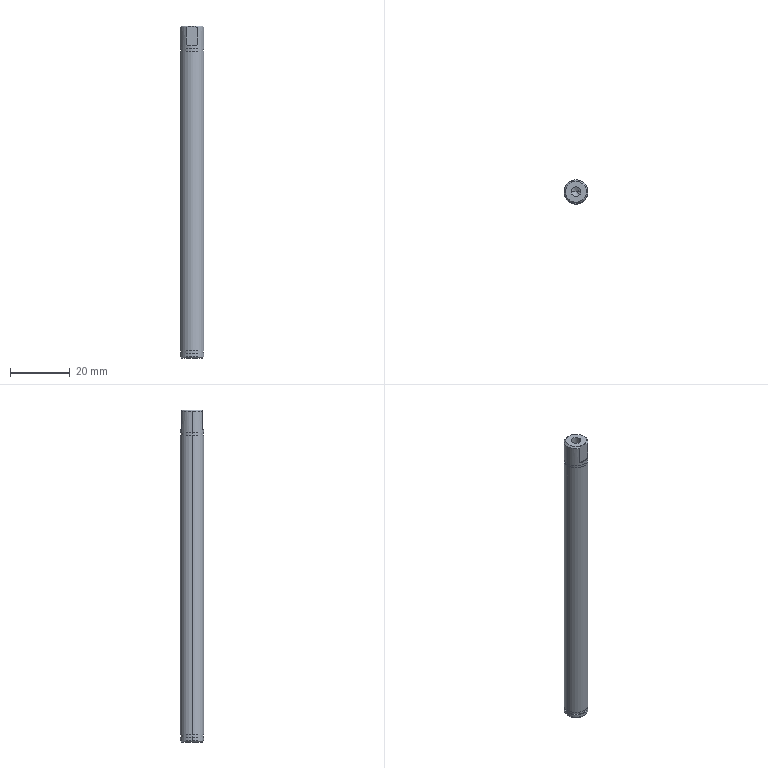Part | STEP file | 11-FG-B06911 | 1 solid | 29 faces | box 8 x 8 x 111 mm | volume 5459 mm3 | cylinder 12 | plane 10 | cone 7 | commonest cylinder face diameters 8 x6 7.6 x4 3.3 x2
STEP:
#1=CARTESIAN_POINT('',(-1.65,0.,100.9));
#2=VERTEX_POINT('',#1);
#3=CARTESIAN_POINT('',(1.65,0.,100.9));
#4=VERTEX_POINT('',#3);
#5=CARTESIAN_POINT('',(0.,0.,100.9));
#6=DIRECTION('',(0.,0.,1.));
#7=DIRECTION('',(1.,0.,0.));
#8=AXIS2_PLACEMENT_3D('',#5,#6,#7);
#9=CIRCLE('',#8,1.65);
#10=EDGE_CURVE('',#2,#4,#9,.T.);
#11=ORIENTED_EDGE('',*,*,#10,.F.);
#12=CARTESIAN_POINT('',(-1.65,0.,111.));
#13=VERTEX_POINT('',#12);
#14=CARTESIAN_POINT('',(-1.65,0.,111.));
#15=DIRECTION('',(0.,0.,1.));
#16=VECTOR('',#15,1000.);
#17=LINE('',#14,#16);
#18=EDGE_CURVE('',#2,#13,#17,.T.);
#19=ORIENTED_EDGE('',*,*,#18,.T.);
#20=CARTESIAN_POINT('',(1.65,0.,111.));
#21=VERTEX_POINT('',#20);
#22=CARTESIAN_POINT('',(0.,0.,111.));
#23=DIRECTION('',(0.,0.,1.));
#24=DIRECTION('',(1.,0.,0.));
#25=AXIS2_PLACEMENT_3D('',#22,#23,#24);
#26=CIRCLE('',#25,1.65);
#27=EDGE_CURVE('',#13,#21,#26,.T.);
#28=ORIENTED_EDGE('',*,*,#27,.T.);
#29=CARTESIAN_POINT('',(1.65,0.,111.));
#30=DIRECTION('',(0.,0.,1.));
#31=VECTOR('',#30,1000.);
#32=LINE('',#29,#31);
#33=EDGE_CURVE('',#4,#21,#32,.T.);
#34=ORIENTED_EDGE('',*,*,#33,.F.);
#35=EDGE_LOOP('',(#11,#19,#28,#34));
#36=FACE_OUTER_BOUND('',#35,.T.);
#37=CARTESIAN_POINT('',(0.,0.,111.));
#38=DIRECTION('',(0.,0.,1.));
#39=DIRECTION('',(1.,0.,0.));
#40=AXIS2_PLACEMENT_3D('',#37,#38,#39);
#41=CYLINDRICAL_SURFACE('',#40,1.65);
#42=ADVANCED_FACE('',(#36),#41,.F.);
#43=CARTESIAN_POINT('',(0.,0.,99.909));
#44=VERTEX_POINT('',#43);
#45=CARTESIAN_POINT('',(1.65,0.,100.9));
#46=DIRECTION('',(0.8572,0.,0.515));
#47=VECTOR('',#46,1000.);
#48=LINE('',#45,#47);
#49=EDGE_CURVE('',#44,#4,#48,.T.);
#50=ORIENTED_EDGE('',*,*,#49,.F.);
#51=CARTESIAN_POINT('',(-1.65,0.,100.9));
#52=DIRECTION('',(-0.8572,0.,0.515));
#53=VECTOR('',#52,1000.);
#54=LINE('',#51,#53);
#55=EDGE_CURVE('',#44,#2,#54,.T.);
#56=ORIENTED_EDGE('',*,*,#55,.T.);
#57=ORIENTED_EDGE('',*,*,#10,.T.);
#58=EDGE_LOOP('',(#50,#56,#57));
#59=FACE_OUTER_BOUND('',#58,.T.);
#60=CARTESIAN_POINT('',(0.,0.,100.9));
#61=DIRECTION('',(0.,0.,1.));
#62=DIRECTION('',(1.,0.,0.));
#63=AXIS2_PLACEMENT_3D('',#60,#61,#62);
#64=CONICAL_SURFACE('',#63,1.65,1.03);
#65=ADVANCED_FACE('',(#59),#64,.F.);
#66=CARTESIAN_POINT('',(1.936,3.5,110.5));
#67=VERTEX_POINT('',#66);
#68=CARTESIAN_POINT('',(4.,0.,110.5));
#69=VERTEX_POINT('',#68);
#70=CARTESIAN_POINT('',(0.,0.,110.5));
#71=DIRECTION('',(0.,0.,-1.));
#72=DIRECTION('',(1.,0.,0.));
#73=AXIS2_PLACEMENT_3D('',#70,#71,#72);
#74=CIRCLE('',#73,4.);
#75=EDGE_CURVE('',#67,#69,#74,.T.);
#76=ORIENTED_EDGE('',*,*,#75,.T.);
#77=CARTESIAN_POINT('',(4.,0.,103.45));
#78=VERTEX_POINT('',#77);
#79=CARTESIAN_POINT('',(4.,0.,111.));
#80=DIRECTION('',(0.,0.,-1.));
#81=VECTOR('',#80,1000.);
#82=LINE('',#79,#81);
#83=EDGE_CURVE('',#69,#78,#82,.T.);
#84=ORIENTED_EDGE('',*,*,#83,.T.);
#85=CARTESIAN_POINT('',(-4.,0.,103.45));
#86=VERTEX_POINT('',#85);
#87=CARTESIAN_POINT('',(0.,0.,103.45));
#88=DIRECTION('',(0.,0.,1.));
#89=DIRECTION('',(1.,0.,0.));
#90=AXIS2_PLACEMENT_3D('',#87,#88,#89);
#91=CIRCLE('',#90,4.);
#92=EDGE_CURVE('',#78,#86,#91,.T.);
#93=ORIENTED_EDGE('',*,*,#92,.T.);
#94=CARTESIAN_POINT('',(-4.,0.,110.5));
#95=VERTEX_POINT('',#94);
#96=CARTESIAN_POINT('',(-4.,0.,111.));
#97=DIRECTION('',(0.,0.,-1.));
#98=VECTOR('',#97,1000.);
#99=LINE('',#96,#98);
#100=EDGE_CURVE('',#95,#86,#99,.T.);
#101=ORIENTED_EDGE('',*,*,#100,.F.);
#102=CARTESIAN_POINT('',(-1.936,3.5,110.5));
#103=VERTEX_POINT('',#102);
#104=CARTESIAN_POINT('',(0.,0.,110.5));
#105=DIRECTION('',(0.,0.,-1.));
#106=DIRECTION('',(1.,0.,0.));
#107=AXIS2_PLACEMENT_3D('',#104,#105,#106);
#108=CIRCLE('',#107,4.);
#109=EDGE_CURVE('',#95,#103,#108,.T.);
#110=ORIENTED_EDGE('',*,*,#109,.T.);
#111=CARTESIAN_POINT('',(-1.936,3.5,104.5));
#112=VERTEX_POINT('',#111);
#113=CARTESIAN_POINT('',(-1.936,3.5,104.5));
#114=DIRECTION('',(0.,0.,1.));
#115=VECTOR('',#114,1000.);
#116=LINE('',#113,#115);
#117=EDGE_CURVE('',#112,#103,#116,.T.);
#118=ORIENTED_EDGE('',*,*,#117,.F.);
#119=CARTESIAN_POINT('',(1.936,3.5,104.5));
#120=VERTEX_POINT('',#119);
#121=CARTESIAN_POINT('',(0.,0.,104.5));
#122=DIRECTION('',(0.,0.,1.));
#123=DIRECTION('',(1.,0.,0.));
#124=AXIS2_PLACEMENT_3D('',#121,#122,#123);
#125=CIRCLE('',#124,4.);
#126=EDGE_CURVE('',#120,#112,#125,.T.);
#127=ORIENTED_EDGE('',*,*,#126,.F.);
#128=CARTESIAN_POINT('',(1.936,3.5,104.5));
#129=DIRECTION('',(0.,0.,1.));
#130=VECTOR('',#129,1000.);
#131=LINE('',#128,#130);
#132=EDGE_CURVE('',#120,#67,#131,.T.);
#133=ORIENTED_EDGE('',*,*,#132,.T.);
#134=EDGE_LOOP('',(#76,#84,#93,#101,#110,#118,#127,#133));
#135=FACE_OUTER_BOUND('',#134,.T.);
#136=CARTESIAN_POINT('',(0.,0.,111.));
#137=DIRECTION('',(0.,0.,-1.));
#138=DIRECTION('',(-1.,0.,0.));
#139=AXIS2_PLACEMENT_3D('',#136,#137,#138);
#140=CYLINDRICAL_SURFACE('',#139,4.);
#141=ADVANCED_FACE('',(#135),#140,.T.);
#142=CARTESIAN_POINT('',(-3.5,0.,111.));
#143=VERTEX_POINT('',#142);
#144=CARTESIAN_POINT('',(0.,-3.5,111.));
#145=VERTEX_POINT('',#144);
#146=CARTESIAN_POINT('',(0.,0.,111.));
#147=DIRECTION('',(0.,0.,1.));
#148=DIRECTION('',(1.,0.,0.));
#149=AXIS2_PLACEMENT_3D('',#146,#147,#148);
#150=CIRCLE('',#149,3.5);
#151=EDGE_CURVE('',#143,#145,#150,.T.);
#152=ORIENTED_EDGE('',*,*,#151,.F.);
#153=CARTESIAN_POINT('',(-3.5,0.,111.));
#154=DIRECTION('',(-0.7071,0.,-0.7071));
#155=VECTOR('',#154,1000.);
#156=LINE('',#153,#155);
#157=EDGE_CURVE('',#143,#95,#156,.T.);
#158=ORIENTED_EDGE('',*,*,#157,.T.);
#159=CARTESIAN_POINT('',(-1.936,-3.5,110.5));
#160=VERTEX_POINT('',#159);
#161=CARTESIAN_POINT('',(0.,0.,110.5));
#162=DIRECTION('',(0.,0.,-1.));
#163=DIRECTION('',(1.,0.,0.));
#164=AXIS2_PLACEMENT_3D('',#161,#162,#163);
#165=CIRCLE('',#164,4.);
#166=EDGE_CURVE('',#160,#95,#165,.T.);
#167=ORIENTED_EDGE('',*,*,#166,.F.);
#168=CARTESIAN_POINT('',(0.,-3.5,111.));
#169=CARTESIAN_POINT('',(-0.3397,-3.5,111.));
#170=CARTESIAN_POINT('',(-0.6719,-3.5,110.95));
#171=CARTESIAN_POINT('',(-1.318,-3.5,110.773));
#172=CARTESIAN_POINT('',(-1.635,-3.5,110.646));
#173=CARTESIAN_POINT('',(-1.936,-3.5,110.5));
#174=B_SPLINE_CURVE_WITH_KNOTS('',3,(#168,#169,#170,#171,#172,#173),.UNSPECIFIED.,.F.,.F.,(4,2,4),(0.004275,0.005275,0.006275),.UNSPECIFIED.);
#175=EDGE_CURVE('',#145,#160,#174,.T.);
#176=ORIENTED_EDGE('',*,*,#175,.F.);
#177=EDGE_LOOP('',(#152,#158,#167,#176));
#178=FACE_OUTER_BOUND('',#177,.T.);
#179=CARTESIAN_POINT('',(0.,0.,111.));
#180=DIRECTION('',(0.,0.,-1.));
#181=DIRECTION('',(-1.,0.,0.));
#182=AXIS2_PLACEMENT_3D('',#179,#180,#181);
#183=CONICAL_SURFACE('',#182,3.5,0.7854);
#184=ADVANCED_FACE('',(#178),#183,.T.);
#185=CARTESIAN_POINT('',(-3.8,0.,103.45));
#186=VERTEX_POINT('',#185);
#187=CARTESIAN_POINT('',(3.8,0.,103.45));
#188=VERTEX_POINT('',#187);
#189=CARTESIAN_POINT('',(0.,0.,103.45));
#190=DIRECTION('',(0.,0.,-1.));
#191=DIRECTION('',(-1.,0.,0.));
#192=AXIS2_PLACEMENT_3D('',#189,#190,#191);
#193=CIRCLE('',#192,3.8);
#194=EDGE_CURVE('',#186,#188,#193,.T.);
#195=ORIENTED_EDGE('',*,*,#194,.T.);
#196=CARTESIAN_POINT('',(3.8,0.,102.55));
#197=VERTEX_POINT('',#196);
#198=CARTESIAN_POINT('',(3.8,0.,-0.6389));
#199=DIRECTION('',(0.,0.,-1.));
#200=VECTOR('',#199,1000.);
#201=LINE('',#198,#200);
#202=EDGE_CURVE('',#188,#197,#201,.T.);
#203=ORIENTED_EDGE('',*,*,#202,.T.);
#204=CARTESIAN_POINT('',(-3.8,0.,102.55));
#205=VERTEX_POINT('',#204);
#206=CARTESIAN_POINT('',(0.,0.,102.55));
#207=DIRECTION('',(0.,0.,-1.));
#208=DIRECTION('',(-1.,0.,0.));
#209=AXIS2_PLACEMENT_3D('',#206,#207,#208);
#210=CIRCLE('',#209,3.8);
#211=EDGE_CURVE('',#205,#197,#210,.T.);
#212=ORIENTED_EDGE('',*,*,#211,.F.);
#213=CARTESIAN_POINT('',(-3.8,0.,-0.6389));
#214=DIRECTION('',(0.,0.,-1.));
#215=VECTOR('',#214,1000.);
#216=LINE('',#213,#215);
#217=EDGE_CURVE('',#186,#205,#216,.T.);
#218=ORIENTED_EDGE('',*,*,#217,.F.);
#219=EDGE_LOOP('',(#195,#203,#212,#218));
#220=FACE_OUTER_BOUND('',#219,.T.);
#221=CARTESIAN_POINT('',(0.,0.,-0.6389));
#222=DIRECTION('',(0.,0.,-1.));
#223=DIRECTION('',(-1.,0.,0.));
#224=AXIS2_PLACEMENT_3D('',#221,#222,#223);
#225=CYLINDRICAL_SURFACE('',#224,3.8);
#226=ADVANCED_FACE('',(#220),#225,.T.);
#227=CARTESIAN_POINT('',(-4.,0.,102.55));
#228=VERTEX_POINT('',#227);
#229=CARTESIAN_POINT('',(4.,0.,102.55));
#230=VERTEX_POINT('',#229);
#231=CARTESIAN_POINT('',(0.,0.,102.55));
#232=DIRECTION('',(0.,0.,-1.));
#233=DIRECTION('',(-1.,0.,0.));
#234=AXIS2_PLACEMENT_3D('',#231,#232,#233);
#235=CIRCLE('',#234,4.);
#236=EDGE_CURVE('',#228,#230,#235,.T.);
#237=ORIENTED_EDGE('',*,*,#236,.T.);
#238=CARTESIAN_POINT('',(4.,0.,2.45));
#239=VERTEX_POINT('',#238);
#240=CARTESIAN_POINT('',(4.,0.,111.));
#241=DIRECTION('',(0.,0.,-1.));
#242=VECTOR('',#241,1000.);
#243=LINE('',#240,#242);
#244=EDGE_CURVE('',#230,#239,#243,.T.);
#245=ORIENTED_EDGE('',*,*,#244,.T.);
#246=CARTESIAN_POINT('',(-4.,0.,2.45));
#247=VERTEX_POINT('',#246);
#248=CARTESIAN_POINT('',(0.,0.,2.45));
#249=DIRECTION('',(0.,0.,1.));
#250=DIRECTION('',(1.,0.,0.));
#251=AXIS2_PLACEMENT_3D('',#248,#249,#250);
#252=CIRCLE('',#251,4.);
#253=EDGE_CURVE('',#239,#247,#252,.T.);
#254=ORIENTED_EDGE('',*,*,#253,.T.);
#255=CARTESIAN_POINT('',(-4.,0.,111.));
#256=DIRECTION('',(0.,0.,-1.));
#257=VECTOR('',#256,1000.);
#258=LINE('',#255,#257);
#259=EDGE_CURVE('',#228,#247,#258,.T.);
#260=ORIENTED_EDGE('',*,*,#259,.F.);
#261=EDGE_LOOP('',(#237,#245,#254,#260));
#262=FACE_OUTER_BOUND('',#261,.T.);
#263=CARTESIAN_POINT('',(0.,0.,111.));
#264=DIRECTION('',(0.,0.,-1.));
#265=DIRECTION('',(-1.,0.,0.));
#266=AXIS2_PLACEMENT_3D('',#263,#264,#265);
#267=CYLINDRICAL_SURFACE('',#266,4.);
#268=ADVANCED_FACE('',(#262),#267,.T.);
#269=CARTESIAN_POINT('',(-3.8,0.,2.45));
#270=VERTEX_POINT('',#269);
#271=CARTESIAN_POINT('',(3.8,0.,2.45));
#272=VERTEX_POINT('',#271);
#273=CARTESIAN_POINT('',(0.,0.,2.45));
#274=DIRECTION('',(0.,0.,-1.));
#275=DIRECTION('',(-1.,0.,0.));
#276=AXIS2_PLACEMENT_3D('',#273,#274,#275);
#277=CIRCLE('',#276,3.8);
#278=EDGE_CURVE('',#270,#272,#277,.T.);
#279=ORIENTED_EDGE('',*,*,#278,.T.);
#280=CARTESIAN_POINT('',(3.8,0.,1.55));
#281=VERTEX_POINT('',#280);
#282=CARTESIAN_POINT('',(3.8,0.,-0.6389));
#283=DIRECTION('',(0.,0.,-1.));
#284=VECTOR('',#283,1000.);
#285=LINE('',#282,#284);
#286=EDGE_CURVE('',#272,#281,#285,.T.);
#287=ORIENTED_EDGE('',*,*,#286,.T.);
#288=CARTESIAN_POINT('',(-3.8,0.,1.55));
#289=VERTEX_POINT('',#288);
#290=CARTESIAN_POINT('',(0.,0.,1.55));
#291=DIRECTION('',(0.,0.,-1.));
#292=DIRECTION('',(-1.,0.,0.));
#293=AXIS2_PLACEMENT_3D('',#290,#291,#292);
#294=CIRCLE('',#293,3.8);
#295=EDGE_CURVE('',#289,#281,#294,.T.);
#296=ORIENTED_EDGE('',*,*,#295,.F.);
#297=CARTESIAN_POINT('',(-3.8,0.,-0.6389));
#298=DIRECTION('',(0.,0.,-1.));
#299=VECTOR('',#298,1000.);
#300=LINE('',#297,#299);
#301=EDGE_CURVE('',#270,#289,#300,.T.);
#302=ORIENTED_EDGE('',*,*,#301,.F.);
#303=EDGE_LOOP('',(#279,#287,#296,#302));
#304=FACE_OUTER_BOUND('',#303,.T.);
#305=CARTESIAN_POINT('',(0.,0.,-0.6389));
#306=DIRECTION('',(0.,0.,-1.));
#307=DIRECTION('',(-1.,0.,0.));
#308=AXIS2_PLACEMENT_3D('',#305,#306,#307);
#309=CYLINDRICAL_SURFACE('',#308,3.8);
#310=ADVANCED_FACE('',(#304),#309,.T.);
#311=CARTESIAN_POINT('',(-3.5,0.,0.));
#312=VERTEX_POINT('',#311);
#313=CARTESIAN_POINT('',(3.5,0.,0.));
#314=VERTEX_POINT('',#313);
#315=CARTESIAN_POINT('',(0.,0.,0.));
#316=DIRECTION('',(0.,0.,-1.));
#317=DIRECTION('',(1.,0.,0.));
#318=AXIS2_PLACEMENT_3D('',#315,#316,#317);
#319=CIRCLE('',#318,3.5);
#320=EDGE_CURVE('',#312,#314,#319,.T.);
#321=ORIENTED_EDGE('',*,*,#320,.F.);
#322=CARTESIAN_POINT('',(-4.,0.,0.5));
#323=VERTEX_POINT('',#322);
#324=CARTESIAN_POINT('',(-4.,0.,0.5));
#325=DIRECTION('',(-0.7071,0.,0.7071));
#326=VECTOR('',#325,1000.);
#327=LINE('',#324,#326);
#328=EDGE_CURVE('',#312,#323,#327,.T.);
#329=ORIENTED_EDGE('',*,*,#328,.T.);
#330=CARTESIAN_POINT('',(4.,0.,0.5));
#331=VERTEX_POINT('',#330);
#332=CARTESIAN_POINT('',(0.,0.,0.5));
#333=DIRECTION('',(0.,0.,1.));
#334=DIRECTION('',(1.,0.,0.));
#335=AXIS2_PLACEMENT_3D('',#332,#333,#334);
#336=CIRCLE('',#335,4.);
#337=EDGE_CURVE('',#331,#323,#336,.T.);
#338=ORIENTED_EDGE('',*,*,#337,.F.);
#339=CARTESIAN_POINT('',(4.,0.,0.5));
#340=DIRECTION('',(0.7071,0.,0.7071));
#341=VECTOR('',#340,1000.);
#342=LINE('',#339,#341);
#343=EDGE_CURVE('',#314,#331,#342,.T.);
#344=ORIENTED_EDGE('',*,*,#343,.F.);
#345=EDGE_LOOP('',(#321,#329,#338,#344));
#346=FACE_OUTER_BOUND('',#345,.T.);
#347=CARTESIAN_POINT('',(0.,0.,0.5));
#348=DIRECTION('',(0.,0.,1.));
#349=DIRECTION('',(1.,0.,0.));
#350=AXIS2_PLACEMENT_3D('',#347,#348,#349);
#351=CONICAL_SURFACE('',#350,4.,0.7854);
#352=ADVANCED_FACE('',(#346),#351,.T.);
#353=CARTESIAN_POINT('',(-4.,0.,1.55));
#354=VERTEX_POINT('',#353);
#355=CARTESIAN_POINT('',(4.,0.,1.55));
#356=VERTEX_POINT('',#355);
#357=CARTESIAN_POINT('',(0.,0.,1.55));
#358=DIRECTION('',(0.,0.,-1.));
#359=DIRECTION('',(-1.,0.,0.));
#360=AXIS2_PLACEMENT_3D('',#357,#358,#359);
#361=CIRCLE('',#360,4.);
#362=EDGE_CURVE('',#354,#356,#361,.T.);
#363=ORIENTED_EDGE('',*,*,#362,.T.);
#364=CARTESIAN_POINT('',(4.,0.,111.));
#365=DIRECTION('',(0.,0.,-1.));
#366=VECTOR('',#365,1000.);
#367=LINE('',#364,#366);
#368=EDGE_CURVE('',#356,#331,#367,.T.);
#369=ORIENTED_EDGE('',*,*,#368,.T.);
#370=ORIENTED_EDGE('',*,*,#337,.T.);
#371=CARTESIAN_POINT('',(-4.,0.,111.));
#372=DIRECTION('',(0.,0.,-1.));
#373=VECTOR('',#372,1000.);
#374=LINE('',#371,#373);
#375=EDGE_CURVE('',#354,#323,#374,.T.);
#376=ORIENTED_EDGE('',*,*,#375,.F.);
#377=EDGE_LOOP('',(#363,#369,#370,#376));
#378=FACE_OUTER_BOUND('',#377,.T.);
#379=CARTESIAN_POINT('',(0.,0.,111.));
#380=DIRECTION('',(0.,0.,-1.));
#381=DIRECTION('',(-1.,0.,0.));
#382=AXIS2_PLACEMENT_3D('',#379,#380,#381);
#383=CYLINDRICAL_SURFACE('',#382,4.);
#384=ADVANCED_FACE('',(#378),#383,.T.);
#385=CARTESIAN_POINT('',(1.936,-3.5,110.5));
#386=VERTEX_POINT('',#385);
#387=CARTESIAN_POINT('',(1.936,-3.5,110.5));
#388=CARTESIAN_POINT('',(1.786,-3.5,110.573));
#389=CARTESIAN_POINT('',(1.633,-3.5,110.641));
#390=CARTESIAN_POINT('',(1.318,-3.5,110.763));
#391=CARTESIAN_POINT('',(1.157,-3.5,110.817));
#392=CARTESIAN_POINT('',(0.6708,-3.5,110.95));
#393=CARTESIAN_POINT('',(0.3398,-3.5,111.));
#394=CARTESIAN_POINT('',(0.,-3.5,111.));
#395=B_SPLINE_CURVE_WITH_KNOTS('',3,(#387,#388,#389,#390,#391,#392,#393,#394),.UNSPECIFIED.,.F.,.F.,(4,2,2,4),(0.002275,0.002775,0.003275,0.004275),.UNSPECIFIED.);
#396=EDGE_CURVE('',#386,#145,#395,.T.);
#397=ORIENTED_EDGE('',*,*,#396,.F.);
#398=CARTESIAN_POINT('',(0.,0.,110.5));
#399=DIRECTION('',(0.,0.,-1.));
#400=DIRECTION('',(1.,0.,0.));
#401=AXIS2_PLACEMENT_3D('',#398,#399,#400);
#402=CIRCLE('',#401,4.);
#403=EDGE_CURVE('',#69,#386,#402,.T.);
#404=ORIENTED_EDGE('',*,*,#403,.F.);
#405=ORIENTED_EDGE('',*,*,#75,.F.);
#406=CARTESIAN_POINT('',(0.,3.5,111.));
#407=VERTEX_POINT('',#406);
#408=CARTESIAN_POINT('',(0.,3.5,111.));
#409=CARTESIAN_POINT('',(0.3398,3.5,111.));
#410=CARTESIAN_POINT('',(0.6708,3.5,110.95));
#411=CARTESIAN_POINT('',(1.157,3.5,110.817));
#412=CARTESIAN_POINT('',(1.318,3.5,110.763));
#413=CARTESIAN_POINT('',(1.633,3.5,110.641));
#414=CARTESIAN_POINT('',(1.786,3.5,110.573));
#415=CARTESIAN_POINT('',(1.936,3.5,110.5));
#416=B_SPLINE_CURVE_WITH_KNOTS('',3,(#408,#409,#410,#411,#412,#413,#414,#415),.UNSPECIFIED.,.F.,.F.,(4,2,2,4),(0.004539,0.00554,0.00604,0.006541),.UNSPECIFIED.);
#417=EDGE_CURVE('',#407,#67,#416,.T.);
#418=ORIENTED_EDGE('',*,*,#417,.F.);
#419=CARTESIAN_POINT('',(0.,0.,111.));
#420=DIRECTION('',(0.,0.,1.));
#421=DIRECTION('',(1.,0.,0.));
#422=AXIS2_PLACEMENT_3D('',#419,#420,#421);
#423=CIRCLE('',#422,3.5);
#424=EDGE_CURVE('',#145,#407,#423,.T.);
#425=ORIENTED_EDGE('',*,*,#424,.F.);
#426=EDGE_LOOP('',(#397,#404,#405,#418,#425));
#427=FACE_OUTER_BOUND('',#426,.T.);
#428=CARTESIAN_POINT('',(0.,0.,111.));
#429=DIRECTION('',(0.,0.,-1.));
#430=DIRECTION('',(-1.,0.,0.));
#431=AXIS2_PLACEMENT_3D('',#428,#429,#430);
#432=CONICAL_SURFACE('',#431,3.5,0.7854);
#433=ADVANCED_FACE('',(#427),#432,.T.);
#434=ORIENTED_EDGE('',*,*,#368,.F.);
#435=CARTESIAN_POINT('',(0.,0.,1.55));
#436=DIRECTION('',(0.,0.,-1.));
#437=DIRECTION('',(-1.,0.,0.));
#438=AXIS2_PLACEMENT_3D('',#435,#436,#437);
#439=CIRCLE('',#438,4.);
#440=EDGE_CURVE('',#356,#354,#439,.T.);
#441=ORIENTED_EDGE('',*,*,#440,.T.);
#442=ORIENTED_EDGE('',*,*,#375,.T.);
#443=CARTESIAN_POINT('',(0.,0.,0.5));
#444=DIRECTION('',(0.,0.,1.));
#445=DIRECTION('',(1.,0.,0.));
#446=AXIS2_PLACEMENT_3D('',#443,#444,#445);
#447=CIRCLE('',#446,4.);
#448=EDGE_CURVE('',#323,#331,#447,.T.);
#449=ORIENTED_EDGE('',*,*,#448,.T.);
#450=EDGE_LOOP('',(#434,#441,#442,#449));
#451=FACE_OUTER_BOUND('',#450,.T.);
#452=CARTESIAN_POINT('',(0.,0.,111.));
#453=DIRECTION('',(0.,0.,-1.));
#454=DIRECTION('',(-1.,0.,0.));
#455=AXIS2_PLACEMENT_3D('',#452,#453,#454);
#456=CYLINDRICAL_SURFACE('',#455,4.);
#457=ADVANCED_FACE('',(#451),#456,.T.);
#458=CARTESIAN_POINT('',(0.,0.,0.));
#459=DIRECTION('',(0.,0.,-1.));
#460=DIRECTION('',(1.,0.,0.));
#461=AXIS2_PLACEMENT_3D('',#458,#459,#460);
#462=CIRCLE('',#461,3.5);
#463=EDGE_CURVE('',#314,#312,#462,.T.);
#464=ORIENTED_EDGE('',*,*,#463,.T.);
#465=ORIENTED_EDGE('',*,*,#320,.T.);
#466=EDGE_LOOP('',(#464,#465));
#467=FACE_OUTER_BOUND('',#466,.T.);
#468=CARTESIAN_POINT('',(0.,0.,0.));
#469=DIRECTION('',(0.,0.,1.));
#470=DIRECTION('',(1.,0.,0.));
#471=AXIS2_PLACEMENT_3D('',#468,#469,#470);
#472=PLANE('',#471);
#473=ADVANCED_FACE('',(#467),#472,.F.);
#474=ORIENTED_EDGE('',*,*,#328,.F.);
#475=ORIENTED_EDGE('',*,*,#463,.F.);
#476=ORIENTED_EDGE('',*,*,#343,.T.);
#477=ORIENTED_EDGE('',*,*,#448,.F.);
#478=EDGE_LOOP('',(#474,#475,#476,#477));
#479=FACE_OUTER_BOUND('',#478,.T.);
#480=CARTESIAN_POINT('',(0.,0.,0.5));
#481=DIRECTION('',(0.,0.,1.));
#482=DIRECTION('',(1.,0.,0.));
#483=AXIS2_PLACEMENT_3D('',#480,#481,#482);
#484=CONICAL_SURFACE('',#483,4.,0.7854);
#485=ADVANCED_FACE('',(#479),#484,.T.);
#486=ORIENTED_EDGE('',*,*,#295,.T.);
#487=CARTESIAN_POINT('',(0.,0.,1.55));
#488=DIRECTION('',(0.,0.,-1.));
#489=DIRECTION('',(-1.,0.,0.));
#490=AXIS2_PLACEMENT_3D('',#487,#488,#489);
#491=CIRCLE('',#490,3.8);
#492=EDGE_CURVE('',#281,#289,#491,.T.);
#493=ORIENTED_EDGE('',*,*,#492,.T.);
#494=EDGE_LOOP('',(#486,#493));
#495=FACE_BOUND('',#494,.T.);
#496=ORIENTED_EDGE('',*,*,#362,.F.);
#497=ORIENTED_EDGE('',*,*,#440,.F.);
#498=EDGE_LOOP('',(#496,#497));
#499=FACE_OUTER_BOUND('',#498,.T.);
#500=CARTESIAN_POINT('',(0.,6.646,1.55));
#501=DIRECTION('',(0.,0.,-1.));
#502=DIRECTION('',(-1.,0.,0.));
#503=AXIS2_PLACEMENT_3D('',#500,#501,#502);
#504=PLANE('',#503);
#505=ADVANCED_FACE('',(#495,#499),#504,.F.);
#506=ORIENTED_EDGE('',*,*,#278,.F.);
#507=CARTESIAN_POINT('',(0.,0.,2.45));
#508=DIRECTION('',(0.,0.,-1.));
#509=DIRECTION('',(-1.,0.,0.));
#510=AXIS2_PLACEMENT_3D('',#507,#508,#509);
#511=CIRCLE('',#510,3.8);
#512=EDGE_CURVE('',#272,#270,#511,.T.);
#513=ORIENTED_EDGE('',*,*,#512,.F.);
#514=EDGE_LOOP('',(#506,#513));
#515=FACE_BOUND('',#514,.T.);
#516=CARTESIAN_POINT('',(0.,0.,2.45));
#517=DIRECTION('',(0.,0.,1.));
#518=DIRECTION('',(1.,0.,0.));
#519=AXIS2_PLACEMENT_3D('',#516,#517,#518);
#520=CIRCLE('',#519,4.);
#521=EDGE_CURVE('',#247,#239,#520,.T.);
#522=ORIENTED_EDGE('',*,*,#521,.F.);
#523=ORIENTED_EDGE('',*,*,#253,.F.);
#524=EDGE_LOOP('',(#522,#523));
#525=FACE_OUTER_BOUND('',#524,.T.);
#526=CARTESIAN_POINT('',(0.,6.646,2.45));
#527=DIRECTION('',(0.,0.,1.));
#528=DIRECTION('',(1.,0.,0.));
#529=AXIS2_PLACEMENT_3D('',#526,#527,#528);
#530=PLANE('',#529);
#531=ADVANCED_FACE('',(#515,#525),#530,.F.);
#532=ORIENTED_EDGE('',*,*,#286,.F.);
#533=ORIENTED_EDGE('',*,*,#512,.T.);
#534=ORIENTED_EDGE('',*,*,#301,.T.);
#535=ORIENTED_EDGE('',*,*,#492,.F.);
#536=EDGE_LOOP('',(#532,#533,#534,#535));
#537=FACE_OUTER_BOUND('',#536,.T.);
#538=CARTESIAN_POINT('',(0.,0.,-0.6389));
#539=DIRECTION('',(0.,0.,-1.));
#540=DIRECTION('',(-1.,0.,0.));
#541=AXIS2_PLACEMENT_3D('',#538,#539,#540);
#542=CYLINDRICAL_SURFACE('',#541,3.8);
#543=ADVANCED_FACE('',(#537),#542,.T.);
#544=ORIENTED_EDGE('',*,*,#244,.F.);
#545=CARTESIAN_POINT('',(0.,0.,102.55));
#546=DIRECTION('',(0.,0.,-1.));
#547=DIRECTION('',(-1.,0.,0.));
#548=AXIS2_PLACEMENT_3D('',#545,#546,#547);
#549=CIRCLE('',#548,4.);
#550=EDGE_CURVE('',#230,#228,#549,.T.);
#551=ORIENTED_EDGE('',*,*,#550,.T.);
#552=ORIENTED_EDGE('',*,*,#259,.T.);
#553=ORIENTED_EDGE('',*,*,#521,.T.);
#554=EDGE_LOOP('',(#544,#551,#552,#553));
#555=FACE_OUTER_BOUND('',#554,.T.);
#556=CARTESIAN_POINT('',(0.,0.,111.));
#557=DIRECTION('',(0.,0.,-1.));
#558=DIRECTION('',(-1.,0.,0.));
#559=AXIS2_PLACEMENT_3D('',#556,#557,#558);
#560=CYLINDRICAL_SURFACE('',#559,4.);
#561=ADVANCED_FACE('',(#555),#560,.T.);
#562=ORIENTED_EDGE('',*,*,#194,.F.);
#563=CARTESIAN_POINT('',(0.,0.,103.45));
#564=DIRECTION('',(0.,0.,-1.));
#565=DIRECTION('',(-1.,0.,0.));
#566=AXIS2_PLACEMENT_3D('',#563,#564,#565);
#567=CIRCLE('',#566,3.8);
#568=EDGE_CURVE('',#188,#186,#567,.T.);
#569=ORIENTED_EDGE('',*,*,#568,.F.);
#570=EDGE_LOOP('',(#562,#569));
#571=FACE_BOUND('',#570,.T.);
#572=CARTESIAN_POINT('',(0.,0.,103.45));
#573=DIRECTION('',(0.,0.,1.));
#574=DIRECTION('',(1.,0.,0.));
#575=AXIS2_PLACEMENT_3D('',#572,#573,#574);
#576=CIRCLE('',#575,4.);
#577=EDGE_CURVE('',#86,#78,#576,.T.);
#578=ORIENTED_EDGE('',*,*,#577,.F.);
#579=ORIENTED_EDGE('',*,*,#92,.F.);
#580=EDGE_LOOP('',(#578,#579));
#581=FACE_OUTER_BOUND('',#580,.T.);
#582=CARTESIAN_POINT('',(0.,9.482,103.45));
#583=DIRECTION('',(0.,0.,1.));
#584=DIRECTION('',(1.,0.,0.));
#585=AXIS2_PLACEMENT_3D('',#582,#583,#584);
#586=PLANE('',#585);
#587=ADVANCED_FACE('',(#571,#581),#586,.F.);
#588=ORIENTED_EDGE('',*,*,#211,.T.);
#589=CARTESIAN_POINT('',(0.,0.,102.55));
#590=DIRECTION('',(0.,0.,-1.));
#591=DIRECTION('',(-1.,0.,0.));
#592=AXIS2_PLACEMENT_3D('',#589,#590,#591);
#593=CIRCLE('',#592,3.8);
#594=EDGE_CURVE('',#197,#205,#593,.T.);
#595=ORIENTED_EDGE('',*,*,#594,.T.);
#596=EDGE_LOOP('',(#588,#595));
#597=FACE_BOUND('',#596,.T.);
#598=ORIENTED_EDGE('',*,*,#236,.F.);
#599=ORIENTED_EDGE('',*,*,#550,.F.);
#600=EDGE_LOOP('',(#598,#599));
#601=FACE_OUTER_BOUND('',#600,.T.);
#602=CARTESIAN_POINT('',(0.,9.482,102.55));
#603=DIRECTION('',(0.,0.,-1.));
#604=DIRECTION('',(-1.,0.,0.));
#605=AXIS2_PLACEMENT_3D('',#602,#603,#604);
#606=PLANE('',#605);
#607=ADVANCED_FACE('',(#597,#601),#606,.F.);
#608=ORIENTED_EDGE('',*,*,#202,.F.);
#609=ORIENTED_EDGE('',*,*,#568,.T.);
#610=ORIENTED_EDGE('',*,*,#217,.T.);
#611=ORIENTED_EDGE('',*,*,#594,.F.);
#612=EDGE_LOOP('',(#608,#609,#610,#611));
#613=FACE_OUTER_BOUND('',#612,.T.);
#614=CARTESIAN_POINT('',(0.,0.,-0.6389));
#615=DIRECTION('',(0.,0.,-1.));
#616=DIRECTION('',(-1.,0.,0.));
#617=AXIS2_PLACEMENT_3D('',#614,#615,#616);
#618=CYLINDRICAL_SURFACE('',#617,3.8);
#619=ADVANCED_FACE('',(#613),#618,.T.);
#620=CARTESIAN_POINT('',(0.,0.,111.));
#621=DIRECTION('',(0.,0.,1.));
#622=DIRECTION('',(1.,0.,0.));
#623=AXIS2_PLACEMENT_3D('',#620,#621,#622);
#624=CIRCLE('',#623,1.65);
#625=EDGE_CURVE('',#21,#13,#624,.T.);
#626=ORIENTED_EDGE('',*,*,#625,.F.);
#627=ORIENTED_EDGE('',*,*,#27,.F.);
#628=EDGE_LOOP('',(#626,#627));
#629=FACE_BOUND('',#628,.T.);
#630=CARTESIAN_POINT('',(0.,0.,111.));
#631=DIRECTION('',(0.,0.,1.));
#632=DIRECTION('',(1.,0.,0.));
#633=AXIS2_PLACEMENT_3D('',#630,#631,#632);
#634=CIRCLE('',#633,3.5);
#635=EDGE_CURVE('',#407,#143,#634,.T.);
#636=ORIENTED_EDGE('',*,*,#635,.T.);
#637=ORIENTED_EDGE('',*,*,#151,.T.);
#638=ORIENTED_EDGE('',*,*,#424,.T.);
#639=EDGE_LOOP('',(#636,#637,#638));
#640=FACE_OUTER_BOUND('',#639,.T.);
#641=CARTESIAN_POINT('',(0.,0.,111.));
#642=DIRECTION('',(0.,0.,1.));
#643=DIRECTION('',(1.,0.,0.));
#644=AXIS2_PLACEMENT_3D('',#641,#642,#643);
#645=PLANE('',#644);
#646=ADVANCED_FACE('',(#629,#640),#645,.T.);
#647=ORIENTED_EDGE('',*,*,#157,.F.);
#648=ORIENTED_EDGE('',*,*,#635,.F.);
#649=CARTESIAN_POINT('',(-1.936,3.5,110.5));
#650=CARTESIAN_POINT('',(-1.635,3.5,110.646));
#651=CARTESIAN_POINT('',(-1.318,3.5,110.773));
#652=CARTESIAN_POINT('',(-0.6719,3.5,110.95));
#653=CARTESIAN_POINT('',(-0.3397,3.5,111.));
#654=CARTESIAN_POINT('',(0.,3.5,111.));
#655=B_SPLINE_CURVE_WITH_KNOTS('',3,(#649,#650,#651,#652,#653,#654),.UNSPECIFIED.,.F.,.F.,(4,2,4),(0.002539,0.003539,0.004539),.UNSPECIFIED.);
#656=EDGE_CURVE('',#103,#407,#655,.T.);
#657=ORIENTED_EDGE('',*,*,#656,.F.);
#658=ORIENTED_EDGE('',*,*,#109,.F.);
#659=EDGE_LOOP('',(#647,#648,#657,#658));
#660=FACE_OUTER_BOUND('',#659,.T.);
#661=CARTESIAN_POINT('',(0.,0.,111.));
#662=DIRECTION('',(0.,0.,-1.));
#663=DIRECTION('',(-1.,0.,0.));
#664=AXIS2_PLACEMENT_3D('',#661,#662,#663);
#665=CONICAL_SURFACE('',#664,3.5,0.7854);
#666=ADVANCED_FACE('',(#660),#665,.T.);
#667=ORIENTED_EDGE('',*,*,#83,.F.);
#668=ORIENTED_EDGE('',*,*,#403,.T.);
#669=CARTESIAN_POINT('',(1.936,-3.5,104.5));
#670=VERTEX_POINT('',#669);
#671=CARTESIAN_POINT('',(1.936,-3.5,104.5));
#672=DIRECTION('',(0.,0.,1.));
#673=VECTOR('',#672,1000.);
#674=LINE('',#671,#673);
#675=EDGE_CURVE('',#670,#386,#674,.T.);
#676=ORIENTED_EDGE('',*,*,#675,.F.);
#677=CARTESIAN_POINT('',(-1.936,-3.5,104.5));
#678=VERTEX_POINT('',#677);
#679=CARTESIAN_POINT('',(0.,0.,104.5));
#680=DIRECTION('',(0.,0.,1.));
#681=DIRECTION('',(1.,0.,0.));
#682=AXIS2_PLACEMENT_3D('',#679,#680,#681);
#683=CIRCLE('',#682,4.);
#684=EDGE_CURVE('',#678,#670,#683,.T.);
#685=ORIENTED_EDGE('',*,*,#684,.F.);
#686=CARTESIAN_POINT('',(-1.936,-3.5,104.5));
#687=DIRECTION('',(0.,0.,1.));
#688=VECTOR('',#687,1000.);
#689=LINE('',#686,#688);
#690=EDGE_CURVE('',#678,#160,#689,.T.);
#691=ORIENTED_EDGE('',*,*,#690,.T.);
#692=ORIENTED_EDGE('',*,*,#166,.T.);
#693=ORIENTED_EDGE('',*,*,#100,.T.);
#694=ORIENTED_EDGE('',*,*,#577,.T.);
#695=EDGE_LOOP('',(#667,#668,#676,#685,#691,#692,#693,#694));
#696=FACE_OUTER_BOUND('',#695,.T.);
#697=CARTESIAN_POINT('',(0.,0.,111.));
#698=DIRECTION('',(0.,0.,-1.));
#699=DIRECTION('',(-1.,0.,0.));
#700=AXIS2_PLACEMENT_3D('',#697,#698,#699);
#701=CYLINDRICAL_SURFACE('',#700,4.);
#702=ADVANCED_FACE('',(#696),#701,.T.);
#703=ORIENTED_EDGE('',*,*,#55,.F.);
#704=ORIENTED_EDGE('',*,*,#49,.T.);
#705=CARTESIAN_POINT('',(0.,0.,100.9));
#706=DIRECTION('',(0.,0.,1.));
#707=DIRECTION('',(1.,0.,0.));
#708=AXIS2_PLACEMENT_3D('',#705,#706,#707);
#709=CIRCLE('',#708,1.65);
#710=EDGE_CURVE('',#4,#2,#709,.T.);
#711=ORIENTED_EDGE('',*,*,#710,.T.);
#712=EDGE_LOOP('',(#703,#704,#711));
#713=FACE_OUTER_BOUND('',#712,.T.);
#714=CARTESIAN_POINT('',(0.,0.,100.9));
#715=DIRECTION('',(0.,0.,1.));
#716=DIRECTION('',(1.,0.,0.));
#717=AXIS2_PLACEMENT_3D('',#714,#715,#716);
#718=CONICAL_SURFACE('',#717,1.65,1.03);
#719=ADVANCED_FACE('',(#713),#718,.F.);
#720=ORIENTED_EDGE('',*,*,#18,.F.);
#721=ORIENTED_EDGE('',*,*,#710,.F.);
#722=ORIENTED_EDGE('',*,*,#33,.T.);
#723=ORIENTED_EDGE('',*,*,#625,.T.);
#724=EDGE_LOOP('',(#720,#721,#722,#723));
#725=FACE_OUTER_BOUND('',#724,.T.);
#726=CARTESIAN_POINT('',(0.,0.,111.));
#727=DIRECTION('',(0.,0.,1.));
#728=DIRECTION('',(1.,0.,0.));
#729=AXIS2_PLACEMENT_3D('',#726,#727,#728);
#730=CYLINDRICAL_SURFACE('',#729,1.65);
#731=ADVANCED_FACE('',(#725),#730,.F.);
#732=ORIENTED_EDGE('',*,*,#656,.T.);
#733=ORIENTED_EDGE('',*,*,#417,.T.);
#734=ORIENTED_EDGE('',*,*,#132,.F.);
#735=CARTESIAN_POINT('',(-1.936,3.5,104.5));
#736=DIRECTION('',(1.,0.,0.));
#737=VECTOR('',#736,1000.);
#738=LINE('',#735,#737);
#739=EDGE_CURVE('',#112,#120,#738,.T.);
#740=ORIENTED_EDGE('',*,*,#739,.F.);
#741=ORIENTED_EDGE('',*,*,#117,.T.);
#742=EDGE_LOOP('',(#732,#733,#734,#740,#741));
#743=FACE_OUTER_BOUND('',#742,.T.);
#744=CARTESIAN_POINT('',(-1.936,3.5,104.5));
#745=DIRECTION('',(0.,-1.,0.));
#746=DIRECTION('',(1.,0.,0.));
#747=AXIS2_PLACEMENT_3D('',#744,#745,#746);
#748=PLANE('',#747);
#749=ADVANCED_FACE('',(#743),#748,.F.);
#750=ORIENTED_EDGE('',*,*,#126,.T.);
#751=ORIENTED_EDGE('',*,*,#739,.T.);
#752=EDGE_LOOP('',(#750,#751));
#753=FACE_OUTER_BOUND('',#752,.T.);
#754=CARTESIAN_POINT('',(0.,0.,104.5));
#755=DIRECTION('',(0.,0.,1.));
#756=DIRECTION('',(1.,0.,0.));
#757=AXIS2_PLACEMENT_3D('',#754,#755,#756);
#758=PLANE('',#757);
#759=ADVANCED_FACE('',(#753),#758,.T.);
#760=ORIENTED_EDGE('',*,*,#396,.T.);
#761=ORIENTED_EDGE('',*,*,#175,.T.);
#762=ORIENTED_EDGE('',*,*,#690,.F.);
#763=CARTESIAN_POINT('',(-1.936,-3.5,104.5));
#764=DIRECTION('',(-1.,0.,0.));
#765=VECTOR('',#764,1000.);
#766=LINE('',#763,#765);
#767=EDGE_CURVE('',#670,#678,#766,.T.);
#768=ORIENTED_EDGE('',*,*,#767,.F.);
#769=ORIENTED_EDGE('',*,*,#675,.T.);
#770=EDGE_LOOP('',(#760,#761,#762,#768,#769));
#771=FACE_OUTER_BOUND('',#770,.T.);
#772=CARTESIAN_POINT('',(-1.936,-3.5,104.5));
#773=DIRECTION('',(0.,1.,0.));
#774=DIRECTION('',(0.,0.,1.));
#775=AXIS2_PLACEMENT_3D('',#772,#773,#774);
#776=PLANE('',#775);
#777=ADVANCED_FACE('',(#771),#776,.F.);
#778=ORIENTED_EDGE('',*,*,#684,.T.);
#779=ORIENTED_EDGE('',*,*,#767,.T.);
#780=EDGE_LOOP('',(#778,#779));
#781=FACE_OUTER_BOUND('',#780,.T.);
#782=CARTESIAN_POINT('',(0.,0.,104.5));
#783=DIRECTION('',(0.,0.,1.));
#784=DIRECTION('',(1.,0.,0.));
#785=AXIS2_PLACEMENT_3D('',#782,#783,#784);
#786=PLANE('',#785);
#787=ADVANCED_FACE('',(#781),#786,.T.);
#788=CLOSED_SHELL('',(#42,#65,#141,#184,#226,#268,#310,#352,#384,#433,#457,#473,#485,#505,#531,#543,#561,#587,#607,#619,#646,#666,#702,#719,#731,#749,#759,#777,#787));
#789=MANIFOLD_SOLID_BREP('',#788);
#790=CARTESIAN_POINT('',(0.,0.,0.));
#791=DIRECTION('',(0.,0.,1.));
#792=DIRECTION('',(1.,0.,0.));
#793=AXIS2_PLACEMENT_3D('',#790,#791,#792);
#794=(LENGTH_UNIT()NAMED_UNIT(*)SI_UNIT(.MILLI.,.METRE.));
#795=UNCERTAINTY_MEASURE_WITH_UNIT(LENGTH_MEASURE(0.00001),#794,'','');
#796=(NAMED_UNIT(*)PLANE_ANGLE_UNIT()SI_UNIT($,.RADIAN.));
#797=(NAMED_UNIT(*)SI_UNIT($,.STERADIAN.)SOLID_ANGLE_UNIT());
#798=(GEOMETRIC_REPRESENTATION_CONTEXT(3)GLOBAL_UNCERTAINTY_ASSIGNED_CONTEXT((#795))GLOBAL_UNIT_ASSIGNED_CONTEXT((#794,#796,#797))REPRESENTATION_CONTEXT('',''));
#799=ADVANCED_BREP_SHAPE_REPRESENTATION('',(#789,#793),#798);